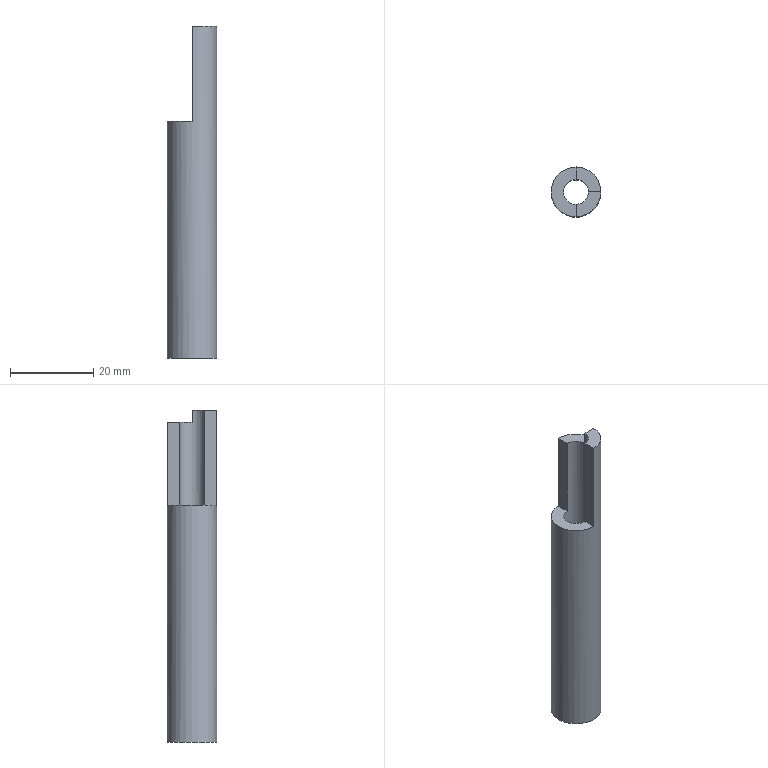Part | NX | features solid 2 | 1 solid | 9 faces | box 12 x 12 x 80 mm | volume 5745 mm3 | plane 7 | cylinder 2 | commonest cylinder face diameters 6.003 x1 12 x1
STEP:
#1=CARTESIAN_POINT('',(4122.094,-795.621,833.716));
#2=VERTEX_POINT('',#1);
#3=CARTESIAN_POINT('',(4122.094,-792.623,833.716));
#4=VERTEX_POINT('',#3);
#5=CARTESIAN_POINT('',(4122.094,-798.623,833.716));
#6=DIRECTION('',(0.,1.,0.));
#7=VECTOR('',#6,1000.);
#8=LINE('',#5,#7);
#9=EDGE_CURVE('',#2,#4,#8,.T.);
#10=ORIENTED_EDGE('',*,*,#9,.T.);
#11=CARTESIAN_POINT('',(4122.094,-792.623,813.716));
#12=VERTEX_POINT('',#11);
#13=CARTESIAN_POINT('',(4122.094,-792.623,836.716));
#14=DIRECTION('',(0.,0.,-1.));
#15=VECTOR('',#14,1000.);
#16=LINE('',#13,#15);
#17=EDGE_CURVE('',#4,#12,#16,.T.);
#18=ORIENTED_EDGE('',*,*,#17,.T.);
#19=CARTESIAN_POINT('',(4122.094,-795.621,813.716));
#20=VERTEX_POINT('',#19);
#21=CARTESIAN_POINT('',(4122.094,-810.623,813.716));
#22=DIRECTION('',(0.,1.,0.));
#23=VECTOR('',#22,1000.);
#24=LINE('',#21,#23);
#25=EDGE_CURVE('',#12,#20,#24,.F.);
#26=ORIENTED_EDGE('',*,*,#25,.T.);
#27=CARTESIAN_POINT('',(4122.094,-795.621,836.716));
#28=DIRECTION('',(0.,0.,-1.));
#29=VECTOR('',#28,1000.);
#30=LINE('',#27,#29);
#31=EDGE_CURVE('',#2,#20,#30,.T.);
#32=ORIENTED_EDGE('',*,*,#31,.F.);
#33=EDGE_LOOP('',(#10,#18,#26,#32));
#34=FACE_BOUND('',#33,.T.);
#35=CARTESIAN_POINT('',(4122.094,-810.623,813.716));
#36=DIRECTION('',(1.,0.,0.));
#37=DIRECTION('',(0.,0.,1.));
#38=AXIS2_PLACEMENT_3D('',#35,#36,#37);
#39=PLANE('',#38);
#40=ADVANCED_FACE('',(#34),#39,.F.);
#41=CARTESIAN_POINT('',(4119.092,-798.623,756.716));
#42=VERTEX_POINT('',#41);
#43=CARTESIAN_POINT('',(4122.094,-798.623,756.716));
#44=DIRECTION('',(0.,0.,1.));
#45=DIRECTION('',(-1.,0.,0.));
#46=AXIS2_PLACEMENT_3D('',#43,#44,#45);
#47=CIRCLE('',#46,3.002);
#48=EDGE_CURVE('',#42,#42,#47,.T.);
#49=ORIENTED_EDGE('',*,*,#48,.T.);
#50=EDGE_LOOP('',(#49));
#51=FACE_BOUND('',#50,.T.);
#52=CARTESIAN_POINT('',(4116.094,-798.623,756.716));
#53=VERTEX_POINT('',#52);
#54=CARTESIAN_POINT('',(4122.094,-798.623,756.716));
#55=DIRECTION('',(0.,0.,1.));
#56=DIRECTION('',(-1.,0.,0.));
#57=AXIS2_PLACEMENT_3D('',#54,#55,#56);
#58=CIRCLE('',#57,6.);
#59=EDGE_CURVE('',#53,#53,#58,.T.);
#60=ORIENTED_EDGE('',*,*,#59,.F.);
#61=EDGE_LOOP('',(#60));
#62=FACE_BOUND('',#61,.T.);
#63=CARTESIAN_POINT('',(4122.094,-798.623,756.716));
#64=DIRECTION('',(0.,0.,-1.));
#65=DIRECTION('',(1.,0.,0.));
#66=AXIS2_PLACEMENT_3D('',#63,#64,#65);
#67=PLANE('',#66);
#68=ADVANCED_FACE('',(#51,#62),#67,.T.);
#69=CARTESIAN_POINT('',(4125.095,-798.623,836.716));
#70=VERTEX_POINT('',#69);
#71=CARTESIAN_POINT('',(4128.094,-798.623,836.716));
#72=VERTEX_POINT('',#71);
#73=CARTESIAN_POINT('',(4122.094,-798.623,836.716));
#74=DIRECTION('',(1.,0.,0.));
#75=VECTOR('',#74,1000.);
#76=LINE('',#73,#75);
#77=EDGE_CURVE('',#70,#72,#76,.T.);
#78=ORIENTED_EDGE('',*,*,#77,.F.);
#79=CARTESIAN_POINT('',(4122.094,-801.624,836.716));
#80=VERTEX_POINT('',#79);
#81=CARTESIAN_POINT('',(4122.094,-798.623,836.716));
#82=DIRECTION('',(0.,0.,-1.));
#83=DIRECTION('',(-1.,0.,0.));
#84=AXIS2_PLACEMENT_3D('',#81,#82,#83);
#85=CIRCLE('',#84,3.002);
#86=EDGE_CURVE('',#70,#80,#85,.T.);
#87=ORIENTED_EDGE('',*,*,#86,.T.);
#88=CARTESIAN_POINT('',(4122.094,-804.623,836.716));
#89=VERTEX_POINT('',#88);
#90=CARTESIAN_POINT('',(4122.094,-810.623,836.716));
#91=DIRECTION('',(0.,1.,0.));
#92=VECTOR('',#91,1000.);
#93=LINE('',#90,#92);
#94=EDGE_CURVE('',#89,#80,#93,.T.);
#95=ORIENTED_EDGE('',*,*,#94,.F.);
#96=CARTESIAN_POINT('',(4122.094,-798.623,836.716));
#97=DIRECTION('',(0.,0.,-1.));
#98=DIRECTION('',(-1.,0.,0.));
#99=AXIS2_PLACEMENT_3D('',#96,#97,#98);
#100=CIRCLE('',#99,6.);
#101=EDGE_CURVE('',#72,#89,#100,.T.);
#102=ORIENTED_EDGE('',*,*,#101,.F.);
#103=EDGE_LOOP('',(#78,#87,#95,#102));
#104=FACE_BOUND('',#103,.T.);
#105=CARTESIAN_POINT('',(4122.094,-798.623,836.716));
#106=DIRECTION('',(0.,0.,1.));
#107=DIRECTION('',(-1.,0.,0.));
#108=AXIS2_PLACEMENT_3D('',#105,#106,#107);
#109=PLANE('',#108);
#110=ADVANCED_FACE('',(#104),#109,.T.);
#111=CARTESIAN_POINT('',(4128.094,-798.623,833.716));
#112=VERTEX_POINT('',#111);
#113=CARTESIAN_POINT('',(4128.094,-798.623,836.716));
#114=DIRECTION('',(0.,0.,-1.));
#115=VECTOR('',#114,1000.);
#116=LINE('',#113,#115);
#117=EDGE_CURVE('',#72,#112,#116,.T.);
#118=ORIENTED_EDGE('',*,*,#117,.F.);
#119=ORIENTED_EDGE('',*,*,#101,.T.);
#120=CARTESIAN_POINT('',(4122.094,-804.623,813.716));
#121=VERTEX_POINT('',#120);
#122=CARTESIAN_POINT('',(4122.094,-804.623,836.716));
#123=DIRECTION('',(0.,0.,-1.));
#124=VECTOR('',#123,1000.);
#125=LINE('',#122,#124);
#126=EDGE_CURVE('',#121,#89,#125,.F.);
#127=ORIENTED_EDGE('',*,*,#126,.F.);
#128=CARTESIAN_POINT('',(4122.094,-798.623,813.716));
#129=DIRECTION('',(0.,0.,-1.));
#130=DIRECTION('',(1.,0.,0.));
#131=AXIS2_PLACEMENT_3D('',#128,#129,#130);
#132=CIRCLE('',#131,6.);
#133=EDGE_CURVE('',#12,#121,#132,.F.);
#134=ORIENTED_EDGE('',*,*,#133,.F.);
#135=ORIENTED_EDGE('',*,*,#17,.F.);
#136=CARTESIAN_POINT('',(4122.094,-798.623,833.716));
#137=DIRECTION('',(0.,0.,1.));
#138=DIRECTION('',(-1.,0.,0.));
#139=AXIS2_PLACEMENT_3D('',#136,#137,#138);
#140=CIRCLE('',#139,6.);
#141=EDGE_CURVE('',#4,#112,#140,.F.);
#142=ORIENTED_EDGE('',*,*,#141,.T.);
#143=EDGE_LOOP('',(#118,#119,#127,#134,#135,#142));
#144=FACE_BOUND('',#143,.T.);
#145=ORIENTED_EDGE('',*,*,#59,.T.);
#146=EDGE_LOOP('',(#145));
#147=FACE_BOUND('',#146,.T.);
#148=CARTESIAN_POINT('',(4122.094,-798.623,836.716));
#149=DIRECTION('',(0.,0.,-1.));
#150=DIRECTION('',(-1.,0.,0.));
#151=AXIS2_PLACEMENT_3D('',#148,#149,#150);
#152=CYLINDRICAL_SURFACE('',#151,6.);
#153=ADVANCED_FACE('',(#144,#147),#152,.T.);
#154=ORIENTED_EDGE('',*,*,#48,.F.);
#155=EDGE_LOOP('',(#154));
#156=FACE_BOUND('',#155,.T.);
#157=ORIENTED_EDGE('',*,*,#86,.F.);
#158=CARTESIAN_POINT('',(4125.095,-798.623,833.716));
#159=VERTEX_POINT('',#158);
#160=CARTESIAN_POINT('',(4125.095,-798.623,836.716));
#161=DIRECTION('',(0.,0.,-1.));
#162=VECTOR('',#161,1000.);
#163=LINE('',#160,#162);
#164=EDGE_CURVE('',#70,#159,#163,.T.);
#165=ORIENTED_EDGE('',*,*,#164,.T.);
#166=CARTESIAN_POINT('',(4122.094,-798.623,833.716));
#167=DIRECTION('',(0.,0.,1.));
#168=DIRECTION('',(-1.,0.,0.));
#169=AXIS2_PLACEMENT_3D('',#166,#167,#168);
#170=CIRCLE('',#169,3.002);
#171=EDGE_CURVE('',#2,#159,#170,.F.);
#172=ORIENTED_EDGE('',*,*,#171,.F.);
#173=ORIENTED_EDGE('',*,*,#31,.T.);
#174=CARTESIAN_POINT('',(4122.094,-801.624,813.716));
#175=VERTEX_POINT('',#174);
#176=CARTESIAN_POINT('',(4122.094,-798.623,813.716));
#177=DIRECTION('',(0.,0.,-1.));
#178=DIRECTION('',(1.,0.,0.));
#179=AXIS2_PLACEMENT_3D('',#176,#177,#178);
#180=CIRCLE('',#179,3.002);
#181=EDGE_CURVE('',#20,#175,#180,.F.);
#182=ORIENTED_EDGE('',*,*,#181,.T.);
#183=CARTESIAN_POINT('',(4122.094,-801.624,836.716));
#184=DIRECTION('',(0.,0.,-1.));
#185=VECTOR('',#184,1000.);
#186=LINE('',#183,#185);
#187=EDGE_CURVE('',#175,#80,#186,.F.);
#188=ORIENTED_EDGE('',*,*,#187,.T.);
#189=EDGE_LOOP('',(#157,#165,#172,#173,#182,#188));
#190=FACE_BOUND('',#189,.T.);
#191=CARTESIAN_POINT('',(4122.094,-798.623,836.716));
#192=DIRECTION('',(0.,0.,-1.));
#193=DIRECTION('',(-1.,0.,0.));
#194=AXIS2_PLACEMENT_3D('',#191,#192,#193);
#195=CYLINDRICAL_SURFACE('',#194,3.002);
#196=ADVANCED_FACE('',(#156,#190),#195,.F.);
#197=ORIENTED_EDGE('',*,*,#126,.T.);
#198=ORIENTED_EDGE('',*,*,#94,.T.);
#199=ORIENTED_EDGE('',*,*,#187,.F.);
#200=CARTESIAN_POINT('',(4122.094,-810.623,813.716));
#201=DIRECTION('',(0.,1.,0.));
#202=VECTOR('',#201,1000.);
#203=LINE('',#200,#202);
#204=EDGE_CURVE('',#175,#121,#203,.F.);
#205=ORIENTED_EDGE('',*,*,#204,.T.);
#206=EDGE_LOOP('',(#197,#198,#199,#205));
#207=FACE_BOUND('',#206,.T.);
#208=CARTESIAN_POINT('',(4122.094,-810.623,813.716));
#209=DIRECTION('',(1.,0.,0.));
#210=DIRECTION('',(0.,0.,1.));
#211=AXIS2_PLACEMENT_3D('',#208,#209,#210);
#212=PLANE('',#211);
#213=ADVANCED_FACE('',(#207),#212,.F.);
#214=ORIENTED_EDGE('',*,*,#133,.T.);
#215=ORIENTED_EDGE('',*,*,#204,.F.);
#216=ORIENTED_EDGE('',*,*,#181,.F.);
#217=ORIENTED_EDGE('',*,*,#25,.F.);
#218=EDGE_LOOP('',(#214,#215,#216,#217));
#219=FACE_BOUND('',#218,.T.);
#220=CARTESIAN_POINT('',(8073.188,-1706.245,813.716));
#221=DIRECTION('',(0.,0.,-1.));
#222=DIRECTION('',(1.,0.,0.));
#223=AXIS2_PLACEMENT_3D('',#220,#221,#222);
#224=PLANE('',#223);
#225=ADVANCED_FACE('',(#219),#224,.F.);
#226=ORIENTED_EDGE('',*,*,#117,.T.);
#227=CARTESIAN_POINT('',(4122.094,-798.623,833.716));
#228=DIRECTION('',(1.,0.,0.));
#229=VECTOR('',#228,1000.);
#230=LINE('',#227,#229);
#231=EDGE_CURVE('',#112,#159,#230,.F.);
#232=ORIENTED_EDGE('',*,*,#231,.T.);
#233=ORIENTED_EDGE('',*,*,#164,.F.);
#234=ORIENTED_EDGE('',*,*,#77,.T.);
#235=EDGE_LOOP('',(#226,#232,#233,#234));
#236=FACE_BOUND('',#235,.T.);
#237=CARTESIAN_POINT('',(4122.094,-798.623,833.716));
#238=DIRECTION('',(0.,-1.,0.));
#239=DIRECTION('',(0.,0.,1.));
#240=AXIS2_PLACEMENT_3D('',#237,#238,#239);
#241=PLANE('',#240);
#242=ADVANCED_FACE('',(#236),#241,.F.);
#243=ORIENTED_EDGE('',*,*,#9,.F.);
#244=ORIENTED_EDGE('',*,*,#171,.T.);
#245=ORIENTED_EDGE('',*,*,#231,.F.);
#246=ORIENTED_EDGE('',*,*,#141,.F.);
#247=EDGE_LOOP('',(#243,#244,#245,#246));
#248=FACE_BOUND('',#247,.T.);
#249=CARTESIAN_POINT('',(8073.188,-1706.245,833.716));
#250=DIRECTION('',(0.,0.,1.));
#251=DIRECTION('',(-1.,0.,0.));
#252=AXIS2_PLACEMENT_3D('',#249,#250,#251);
#253=PLANE('',#252);
#254=ADVANCED_FACE('',(#248),#253,.T.);
#255=CLOSED_SHELL('',(#40,#68,#110,#153,#196,#213,#225,#242,#254));
#256=MANIFOLD_SOLID_BREP('',#255);
#257=(LENGTH_UNIT()NAMED_UNIT(*)SI_UNIT(.MILLI.,.METRE.));
#258=UNCERTAINTY_MEASURE_WITH_UNIT(LENGTH_MEASURE(0.00001),#257,'','');
#259=(NAMED_UNIT(*)PLANE_ANGLE_UNIT()SI_UNIT($,.RADIAN.));
#260=(NAMED_UNIT(*)SI_UNIT($,.STERADIAN.)SOLID_ANGLE_UNIT());
#261=(GEOMETRIC_REPRESENTATION_CONTEXT(3)GLOBAL_UNCERTAINTY_ASSIGNED_CONTEXT((#258))GLOBAL_UNIT_ASSIGNED_CONTEXT((#257,#259,#260))REPRESENTATION_CONTEXT('',''));
#262=ADVANCED_BREP_SHAPE_REPRESENTATION('',(#256),#261);